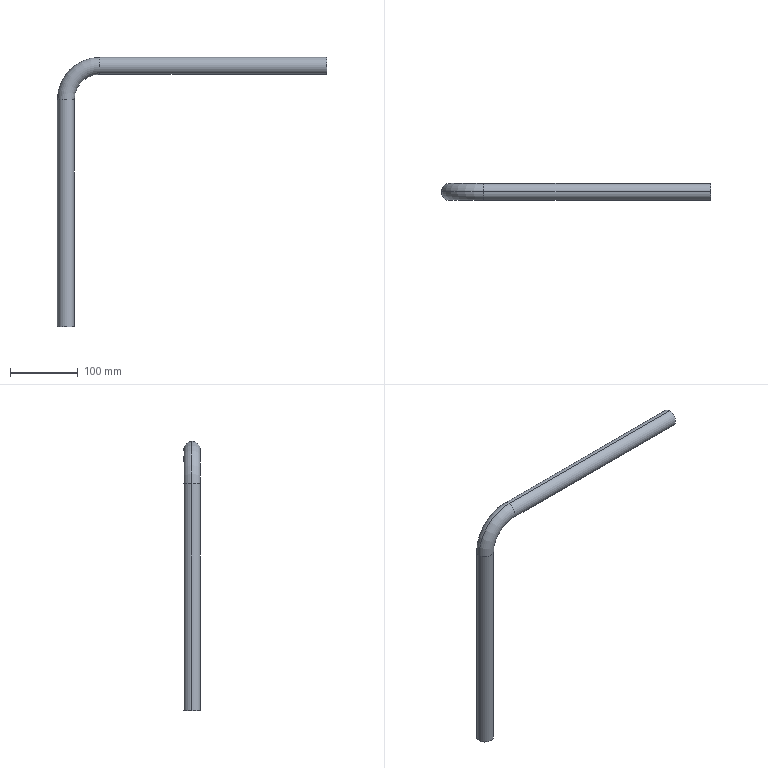Part | STEP file | 护栏90度栏杆_Default<As Machined> | 3 solids | 18 faces | box 397.5 x 25 x 397.5 mm | volume 82894 mm3 | cylinder 8 | plane 6 | torus 4 | commonest cylinder face diameters 22 x4 25 x4
STEP:
#1=CARTESIAN_POINT('',(0.,0.,0.));
#2=DIRECTION('',(0.,0.,1.));
#3=DIRECTION('',(1.,0.,0.));
#4=AXIS2_PLACEMENT_3D('',#1,#2,#3);
#5=CARTESIAN_POINT('',(50.,0.,12.5));
#6=VERTEX_POINT('',#5);
#7=CARTESIAN_POINT('',(50.,0.,-12.5));
#8=VERTEX_POINT('',#7);
#9=CARTESIAN_POINT('',(50.,0.,0.));
#10=DIRECTION('',(-1.,0.,0.));
#11=DIRECTION('',(0.,0.,1.));
#12=AXIS2_PLACEMENT_3D('',#9,#10,#11);
#13=CIRCLE('',#12,12.5);
#14=CARTESIAN_POINT('',(50.,0.,0.));
#15=DIRECTION('',(1.,0.,0.));
#16=DIRECTION('',(0.,0.,-1.));
#17=AXIS2_PLACEMENT_3D('',#14,#15,#16);
#18=CYLINDRICAL_SURFACE('',#17,12.5);
#19=CARTESIAN_POINT('',(3.142,0.));
#20=DIRECTION('',(-1.,0.));
#21=VECTOR('',#20,1.);
#22=LINE('',#19,#21);
#23=(GEOMETRIC_REPRESENTATION_CONTEXT(2)PARAMETRIC_REPRESENTATION_CONTEXT()REPRESENTATION_CONTEXT('',''));
#24=DEFINITIONAL_REPRESENTATION('',(#22),#23);
#25=PCURVE('',#18,#24);
#26=CARTESIAN_POINT('',(50.,0.,0.));
#27=DIRECTION('',(-1.,0.,0.));
#28=DIRECTION('',(0.,0.,1.));
#29=AXIS2_PLACEMENT_3D('',#26,#27,#28);
#30=PLANE('',#29);
#31=CARTESIAN_POINT('',(0.,0.));
#32=DIRECTION('',(1.,0.));
#33=AXIS2_PLACEMENT_2D('',#31,#32);
#34=CIRCLE('',#33,12.5);
#35=(GEOMETRIC_REPRESENTATION_CONTEXT(2)PARAMETRIC_REPRESENTATION_CONTEXT()REPRESENTATION_CONTEXT('',''));
#36=DEFINITIONAL_REPRESENTATION('',(#34),#35);
#37=PCURVE('',#30,#36);
#38=SURFACE_CURVE('',#13,(#25,#37),.PCURVE_S1.);
#39=EDGE_CURVE('',#6,#8,#38,.T.);
#40=ORIENTED_EDGE('',*,*,#39,.F.);
#41=CARTESIAN_POINT('',(385.,0.,12.5));
#42=VERTEX_POINT('',#41);
#43=CARTESIAN_POINT('',(50.,0.,12.5));
#44=DIRECTION('',(1.,0.,0.));
#45=VECTOR('',#44,1.);
#46=LINE('',#43,#45);
#47=CARTESIAN_POINT('',(3.142,0.));
#48=DIRECTION('',(0.,1.));
#49=VECTOR('',#48,1.);
#50=LINE('',#47,#49);
#51=(GEOMETRIC_REPRESENTATION_CONTEXT(2)PARAMETRIC_REPRESENTATION_CONTEXT()REPRESENTATION_CONTEXT('',''));
#52=DEFINITIONAL_REPRESENTATION('',(#50),#51);
#53=PCURVE('',#18,#52);
#54=CARTESIAN_POINT('',(50.,0.,0.));
#55=DIRECTION('',(1.,0.,0.));
#56=DIRECTION('',(0.,0.,-1.));
#57=AXIS2_PLACEMENT_3D('',#54,#55,#56);
#58=CYLINDRICAL_SURFACE('',#57,12.5);
#59=CARTESIAN_POINT('',(3.142,0.));
#60=DIRECTION('',(0.,1.));
#61=VECTOR('',#60,1.);
#62=LINE('',#59,#61);
#63=(GEOMETRIC_REPRESENTATION_CONTEXT(2)PARAMETRIC_REPRESENTATION_CONTEXT()REPRESENTATION_CONTEXT('',''));
#64=DEFINITIONAL_REPRESENTATION('',(#62),#63);
#65=PCURVE('',#58,#64);
#66=SURFACE_CURVE('',#46,(#53,#65),.PCURVE_S1.);
#67=EDGE_CURVE('',#6,#42,#66,.T.);
#68=ORIENTED_EDGE('',*,*,#67,.T.);
#69=CARTESIAN_POINT('',(385.,0.,-12.5));
#70=VERTEX_POINT('',#69);
#71=CARTESIAN_POINT('',(385.,0.,0.));
#72=DIRECTION('',(-1.,0.,0.));
#73=DIRECTION('',(0.,0.,1.));
#74=AXIS2_PLACEMENT_3D('',#71,#72,#73);
#75=CIRCLE('',#74,12.5);
#76=CARTESIAN_POINT('',(3.142,335.));
#77=DIRECTION('',(-1.,0.));
#78=VECTOR('',#77,1.);
#79=LINE('',#76,#78);
#80=(GEOMETRIC_REPRESENTATION_CONTEXT(2)PARAMETRIC_REPRESENTATION_CONTEXT()REPRESENTATION_CONTEXT('',''));
#81=DEFINITIONAL_REPRESENTATION('',(#79),#80);
#82=PCURVE('',#18,#81);
#83=CARTESIAN_POINT('',(385.,0.,0.));
#84=DIRECTION('',(-1.,0.,0.));
#85=DIRECTION('',(0.,0.,1.));
#86=AXIS2_PLACEMENT_3D('',#83,#84,#85);
#87=PLANE('',#86);
#88=CARTESIAN_POINT('',(0.,0.));
#89=DIRECTION('',(1.,0.));
#90=AXIS2_PLACEMENT_2D('',#88,#89);
#91=CIRCLE('',#90,12.5);
#92=(GEOMETRIC_REPRESENTATION_CONTEXT(2)PARAMETRIC_REPRESENTATION_CONTEXT()REPRESENTATION_CONTEXT('',''));
#93=DEFINITIONAL_REPRESENTATION('',(#91),#92);
#94=PCURVE('',#87,#93);
#95=SURFACE_CURVE('',#75,(#82,#94),.PCURVE_S1.);
#96=EDGE_CURVE('',#42,#70,#95,.T.);
#97=ORIENTED_EDGE('',*,*,#96,.T.);
#98=CARTESIAN_POINT('',(50.,0.,-12.5));
#99=DIRECTION('',(1.,0.,0.));
#100=VECTOR('',#99,1.);
#101=LINE('',#98,#100);
#102=CARTESIAN_POINT('',(0.,0.));
#103=DIRECTION('',(0.,1.));
#104=VECTOR('',#103,1.);
#105=LINE('',#102,#104);
#106=(GEOMETRIC_REPRESENTATION_CONTEXT(2)PARAMETRIC_REPRESENTATION_CONTEXT()REPRESENTATION_CONTEXT('',''));
#107=DEFINITIONAL_REPRESENTATION('',(#105),#106);
#108=PCURVE('',#18,#107);
#109=CARTESIAN_POINT('',(6.283,0.));
#110=DIRECTION('',(0.,1.));
#111=VECTOR('',#110,1.);
#112=LINE('',#109,#111);
#113=(GEOMETRIC_REPRESENTATION_CONTEXT(2)PARAMETRIC_REPRESENTATION_CONTEXT()REPRESENTATION_CONTEXT('',''));
#114=DEFINITIONAL_REPRESENTATION('',(#112),#113);
#115=PCURVE('',#58,#114);
#116=SURFACE_CURVE('',#101,(#108,#115),.PCURVE_S1.);
#117=EDGE_CURVE('',#8,#70,#116,.T.);
#118=ORIENTED_EDGE('',*,*,#117,.F.);
#119=EDGE_LOOP('',(#40,#68,#97,#118));
#120=FACE_BOUND('',#119,.T.);
#121=ADVANCED_FACE('',(#120),#18,.T.);
#122=CARTESIAN_POINT('',(50.,0.,-11.));
#123=VERTEX_POINT('',#122);
#124=CARTESIAN_POINT('',(385.,0.,-11.));
#125=VERTEX_POINT('',#124);
#126=CARTESIAN_POINT('',(50.,0.,-11.));
#127=DIRECTION('',(1.,0.,0.));
#128=VECTOR('',#127,1.);
#129=LINE('',#126,#128);
#130=CARTESIAN_POINT('',(50.,0.,0.));
#131=DIRECTION('',(1.,0.,0.));
#132=DIRECTION('',(0.,0.,-1.));
#133=AXIS2_PLACEMENT_3D('',#130,#131,#132);
#134=CYLINDRICAL_SURFACE('',#133,11.);
#135=CARTESIAN_POINT('',(6.283,0.));
#136=DIRECTION('',(0.,1.));
#137=VECTOR('',#136,1.);
#138=LINE('',#135,#137);
#139=(GEOMETRIC_REPRESENTATION_CONTEXT(2)PARAMETRIC_REPRESENTATION_CONTEXT()REPRESENTATION_CONTEXT('',''));
#140=DEFINITIONAL_REPRESENTATION('',(#138),#139);
#141=PCURVE('',#134,#140);
#142=CARTESIAN_POINT('',(50.,0.,0.));
#143=DIRECTION('',(1.,0.,0.));
#144=DIRECTION('',(0.,0.,-1.));
#145=AXIS2_PLACEMENT_3D('',#142,#143,#144);
#146=CYLINDRICAL_SURFACE('',#145,11.);
#147=CARTESIAN_POINT('',(0.,0.));
#148=DIRECTION('',(0.,1.));
#149=VECTOR('',#148,1.);
#150=LINE('',#147,#149);
#151=(GEOMETRIC_REPRESENTATION_CONTEXT(2)PARAMETRIC_REPRESENTATION_CONTEXT()REPRESENTATION_CONTEXT('',''));
#152=DEFINITIONAL_REPRESENTATION('',(#150),#151);
#153=PCURVE('',#146,#152);
#154=SURFACE_CURVE('',#129,(#141,#153),.PCURVE_S1.);
#155=EDGE_CURVE('',#123,#125,#154,.T.);
#156=ORIENTED_EDGE('',*,*,#155,.T.);
#157=CARTESIAN_POINT('',(385.,0.,11.));
#158=VERTEX_POINT('',#157);
#159=CARTESIAN_POINT('',(385.,0.,0.));
#160=DIRECTION('',(-1.,0.,0.));
#161=DIRECTION('',(0.,0.,1.));
#162=AXIS2_PLACEMENT_3D('',#159,#160,#161);
#163=CIRCLE('',#162,11.);
#164=CARTESIAN_POINT('',(9.425,335.));
#165=DIRECTION('',(-1.,0.));
#166=VECTOR('',#165,1.);
#167=LINE('',#164,#166);
#168=(GEOMETRIC_REPRESENTATION_CONTEXT(2)PARAMETRIC_REPRESENTATION_CONTEXT()REPRESENTATION_CONTEXT('',''));
#169=DEFINITIONAL_REPRESENTATION('',(#167),#168);
#170=PCURVE('',#134,#169);
#171=CARTESIAN_POINT('',(0.,0.));
#172=DIRECTION('',(1.,0.));
#173=AXIS2_PLACEMENT_2D('',#171,#172);
#174=CIRCLE('',#173,11.);
#175=(GEOMETRIC_REPRESENTATION_CONTEXT(2)PARAMETRIC_REPRESENTATION_CONTEXT()REPRESENTATION_CONTEXT('',''));
#176=DEFINITIONAL_REPRESENTATION('',(#174),#175);
#177=PCURVE('',#87,#176);
#178=SURFACE_CURVE('',#163,(#170,#177),.PCURVE_S1.);
#179=EDGE_CURVE('',#125,#158,#178,.T.);
#180=ORIENTED_EDGE('',*,*,#179,.T.);
#181=CARTESIAN_POINT('',(50.,0.,11.));
#182=VERTEX_POINT('',#181);
#183=CARTESIAN_POINT('',(50.,0.,11.));
#184=DIRECTION('',(1.,0.,0.));
#185=VECTOR('',#184,1.);
#186=LINE('',#183,#185);
#187=CARTESIAN_POINT('',(3.142,0.));
#188=DIRECTION('',(0.,1.));
#189=VECTOR('',#188,1.);
#190=LINE('',#187,#189);
#191=(GEOMETRIC_REPRESENTATION_CONTEXT(2)PARAMETRIC_REPRESENTATION_CONTEXT()REPRESENTATION_CONTEXT('',''));
#192=DEFINITIONAL_REPRESENTATION('',(#190),#191);
#193=PCURVE('',#134,#192);
#194=CARTESIAN_POINT('',(3.142,0.));
#195=DIRECTION('',(0.,1.));
#196=VECTOR('',#195,1.);
#197=LINE('',#194,#196);
#198=(GEOMETRIC_REPRESENTATION_CONTEXT(2)PARAMETRIC_REPRESENTATION_CONTEXT()REPRESENTATION_CONTEXT('',''));
#199=DEFINITIONAL_REPRESENTATION('',(#197),#198);
#200=PCURVE('',#146,#199);
#201=SURFACE_CURVE('',#186,(#193,#200),.PCURVE_S1.);
#202=EDGE_CURVE('',#182,#158,#201,.T.);
#203=ORIENTED_EDGE('',*,*,#202,.F.);
#204=CARTESIAN_POINT('',(50.,0.,0.));
#205=DIRECTION('',(-1.,0.,0.));
#206=DIRECTION('',(0.,0.,1.));
#207=AXIS2_PLACEMENT_3D('',#204,#205,#206);
#208=CIRCLE('',#207,11.);
#209=CARTESIAN_POINT('',(9.425,0.));
#210=DIRECTION('',(-1.,0.));
#211=VECTOR('',#210,1.);
#212=LINE('',#209,#211);
#213=(GEOMETRIC_REPRESENTATION_CONTEXT(2)PARAMETRIC_REPRESENTATION_CONTEXT()REPRESENTATION_CONTEXT('',''));
#214=DEFINITIONAL_REPRESENTATION('',(#212),#213);
#215=PCURVE('',#134,#214);
#216=CARTESIAN_POINT('',(0.,0.));
#217=DIRECTION('',(1.,0.));
#218=AXIS2_PLACEMENT_2D('',#216,#217);
#219=CIRCLE('',#218,11.);
#220=(GEOMETRIC_REPRESENTATION_CONTEXT(2)PARAMETRIC_REPRESENTATION_CONTEXT()REPRESENTATION_CONTEXT('',''));
#221=DEFINITIONAL_REPRESENTATION('',(#219),#220);
#222=PCURVE('',#30,#221);
#223=SURFACE_CURVE('',#208,(#215,#222),.PCURVE_S1.);
#224=EDGE_CURVE('',#123,#182,#223,.T.);
#225=ORIENTED_EDGE('',*,*,#224,.F.);
#226=EDGE_LOOP('',(#156,#180,#203,#225));
#227=FACE_BOUND('',#226,.F.);
#228=ADVANCED_FACE('',(#227),#134,.F.);
#229=CARTESIAN_POINT('',(385.,0.,0.));
#230=DIRECTION('',(-1.,0.,0.));
#231=DIRECTION('',(0.,0.,1.));
#232=AXIS2_PLACEMENT_3D('',#229,#230,#231);
#233=CIRCLE('',#232,11.);
#234=CARTESIAN_POINT('',(3.142,335.));
#235=DIRECTION('',(-1.,0.));
#236=VECTOR('',#235,1.);
#237=LINE('',#234,#236);
#238=(GEOMETRIC_REPRESENTATION_CONTEXT(2)PARAMETRIC_REPRESENTATION_CONTEXT()REPRESENTATION_CONTEXT('',''));
#239=DEFINITIONAL_REPRESENTATION('',(#237),#238);
#240=PCURVE('',#146,#239);
#241=CARTESIAN_POINT('',(0.,0.));
#242=DIRECTION('',(1.,0.));
#243=AXIS2_PLACEMENT_2D('',#241,#242);
#244=CIRCLE('',#243,11.);
#245=(GEOMETRIC_REPRESENTATION_CONTEXT(2)PARAMETRIC_REPRESENTATION_CONTEXT()REPRESENTATION_CONTEXT('',''));
#246=DEFINITIONAL_REPRESENTATION('',(#244),#245);
#247=PCURVE('',#87,#246);
#248=SURFACE_CURVE('',#233,(#240,#247),.PCURVE_S1.);
#249=EDGE_CURVE('',#158,#125,#248,.T.);
#250=ORIENTED_EDGE('',*,*,#249,.T.);
#251=ORIENTED_EDGE('',*,*,#155,.F.);
#252=CARTESIAN_POINT('',(50.,0.,0.));
#253=DIRECTION('',(-1.,0.,0.));
#254=DIRECTION('',(0.,0.,1.));
#255=AXIS2_PLACEMENT_3D('',#252,#253,#254);
#256=CIRCLE('',#255,11.);
#257=CARTESIAN_POINT('',(3.142,0.));
#258=DIRECTION('',(-1.,0.));
#259=VECTOR('',#258,1.);
#260=LINE('',#257,#259);
#261=(GEOMETRIC_REPRESENTATION_CONTEXT(2)PARAMETRIC_REPRESENTATION_CONTEXT()REPRESENTATION_CONTEXT('',''));
#262=DEFINITIONAL_REPRESENTATION('',(#260),#261);
#263=PCURVE('',#146,#262);
#264=CARTESIAN_POINT('',(0.,0.));
#265=DIRECTION('',(1.,0.));
#266=AXIS2_PLACEMENT_2D('',#264,#265);
#267=CIRCLE('',#266,11.);
#268=(GEOMETRIC_REPRESENTATION_CONTEXT(2)PARAMETRIC_REPRESENTATION_CONTEXT()REPRESENTATION_CONTEXT('',''));
#269=DEFINITIONAL_REPRESENTATION('',(#267),#268);
#270=PCURVE('',#30,#269);
#271=SURFACE_CURVE('',#256,(#263,#270),.PCURVE_S1.);
#272=EDGE_CURVE('',#182,#123,#271,.T.);
#273=ORIENTED_EDGE('',*,*,#272,.F.);
#274=ORIENTED_EDGE('',*,*,#202,.T.);
#275=EDGE_LOOP('',(#250,#251,#273,#274));
#276=FACE_BOUND('',#275,.F.);
#277=ADVANCED_FACE('',(#276),#146,.F.);
#278=ORIENTED_EDGE('',*,*,#67,.F.);
#279=CARTESIAN_POINT('',(50.,0.,0.));
#280=DIRECTION('',(-1.,0.,0.));
#281=DIRECTION('',(0.,0.,1.));
#282=AXIS2_PLACEMENT_3D('',#279,#280,#281);
#283=CIRCLE('',#282,12.5);
#284=CARTESIAN_POINT('',(9.425,0.));
#285=DIRECTION('',(-1.,0.));
#286=VECTOR('',#285,1.);
#287=LINE('',#284,#286);
#288=(GEOMETRIC_REPRESENTATION_CONTEXT(2)PARAMETRIC_REPRESENTATION_CONTEXT()REPRESENTATION_CONTEXT('',''));
#289=DEFINITIONAL_REPRESENTATION('',(#287),#288);
#290=PCURVE('',#58,#289);
#291=CARTESIAN_POINT('',(0.,0.));
#292=DIRECTION('',(1.,0.));
#293=AXIS2_PLACEMENT_2D('',#291,#292);
#294=CIRCLE('',#293,12.5);
#295=(GEOMETRIC_REPRESENTATION_CONTEXT(2)PARAMETRIC_REPRESENTATION_CONTEXT()REPRESENTATION_CONTEXT('',''));
#296=DEFINITIONAL_REPRESENTATION('',(#294),#295);
#297=PCURVE('',#30,#296);
#298=SURFACE_CURVE('',#283,(#290,#297),.PCURVE_S1.);
#299=EDGE_CURVE('',#8,#6,#298,.T.);
#300=ORIENTED_EDGE('',*,*,#299,.F.);
#301=ORIENTED_EDGE('',*,*,#117,.T.);
#302=CARTESIAN_POINT('',(385.,0.,0.));
#303=DIRECTION('',(-1.,0.,0.));
#304=DIRECTION('',(0.,0.,1.));
#305=AXIS2_PLACEMENT_3D('',#302,#303,#304);
#306=CIRCLE('',#305,12.5);
#307=CARTESIAN_POINT('',(9.425,335.));
#308=DIRECTION('',(-1.,0.));
#309=VECTOR('',#308,1.);
#310=LINE('',#307,#309);
#311=(GEOMETRIC_REPRESENTATION_CONTEXT(2)PARAMETRIC_REPRESENTATION_CONTEXT()REPRESENTATION_CONTEXT('',''));
#312=DEFINITIONAL_REPRESENTATION('',(#310),#311);
#313=PCURVE('',#58,#312);
#314=CARTESIAN_POINT('',(0.,0.));
#315=DIRECTION('',(1.,0.));
#316=AXIS2_PLACEMENT_2D('',#314,#315);
#317=CIRCLE('',#316,12.5);
#318=(GEOMETRIC_REPRESENTATION_CONTEXT(2)PARAMETRIC_REPRESENTATION_CONTEXT()REPRESENTATION_CONTEXT('',''));
#319=DEFINITIONAL_REPRESENTATION('',(#317),#318);
#320=PCURVE('',#87,#319);
#321=SURFACE_CURVE('',#306,(#313,#320),.PCURVE_S1.);
#322=EDGE_CURVE('',#70,#42,#321,.T.);
#323=ORIENTED_EDGE('',*,*,#322,.T.);
#324=EDGE_LOOP('',(#278,#300,#301,#323));
#325=FACE_BOUND('',#324,.T.);
#326=ADVANCED_FACE('',(#325),#58,.T.);
#327=ORIENTED_EDGE('',*,*,#179,.T.);
#328=ORIENTED_EDGE('',*,*,#249,.T.);
#329=EDGE_LOOP('',(#327,#328));
#330=FACE_BOUND('',#329,.T.);
#331=ORIENTED_EDGE('',*,*,#322,.F.);
#332=ORIENTED_EDGE('',*,*,#96,.F.);
#333=EDGE_LOOP('',(#331,#332));
#334=FACE_BOUND('',#333,.T.);
#335=ADVANCED_FACE('',(#330,#334),#87,.F.);
#336=ORIENTED_EDGE('',*,*,#224,.F.);
#337=ORIENTED_EDGE('',*,*,#272,.F.);
#338=EDGE_LOOP('',(#336,#337));
#339=FACE_BOUND('',#338,.T.);
#340=ORIENTED_EDGE('',*,*,#299,.T.);
#341=ORIENTED_EDGE('',*,*,#39,.T.);
#342=EDGE_LOOP('',(#340,#341));
#343=FACE_BOUND('',#342,.T.);
#344=ADVANCED_FACE('',(#339,#343),#30,.T.);
#345=CLOSED_SHELL('',(#121,#228,#277,#326,#335,#344));
#346=MANIFOLD_SOLID_BREP('',#345);
#347=CARTESIAN_POINT('',(-12.5,0.,-50.));
#348=VERTEX_POINT('',#347);
#349=CARTESIAN_POINT('',(12.5,0.,-50.));
#350=VERTEX_POINT('',#349);
#351=CARTESIAN_POINT('',(0.,0.,-50.));
#352=DIRECTION('',(0.,0.,-1.));
#353=DIRECTION('',(-1.,0.,0.));
#354=AXIS2_PLACEMENT_3D('',#351,#352,#353);
#355=CIRCLE('',#354,12.5);
#356=CARTESIAN_POINT('',(50.,0.,-50.));
#357=DIRECTION('',(0.,1.,0.));
#358=DIRECTION('',(0.,0.,1.));
#359=AXIS2_PLACEMENT_3D('',#356,#357,#358);
#360=TOROIDAL_SURFACE('',#359,50.,12.5);
#361=CARTESIAN_POINT('',(4.712,0.));
#362=DIRECTION('',(0.,1.));
#363=VECTOR('',#362,1.);
#364=LINE('',#361,#363);
#365=(GEOMETRIC_REPRESENTATION_CONTEXT(2)PARAMETRIC_REPRESENTATION_CONTEXT()REPRESENTATION_CONTEXT('',''));
#366=DEFINITIONAL_REPRESENTATION('',(#364),#365);
#367=PCURVE('',#360,#366);
#368=CARTESIAN_POINT('',(0.,0.,-50.));
#369=DIRECTION('',(0.,0.,-1.));
#370=DIRECTION('',(-1.,0.,0.));
#371=AXIS2_PLACEMENT_3D('',#368,#369,#370);
#372=PLANE('',#371);
#373=CARTESIAN_POINT('',(0.,0.));
#374=DIRECTION('',(1.,0.));
#375=AXIS2_PLACEMENT_2D('',#373,#374);
#376=CIRCLE('',#375,12.5);
#377=(GEOMETRIC_REPRESENTATION_CONTEXT(2)PARAMETRIC_REPRESENTATION_CONTEXT()REPRESENTATION_CONTEXT('',''));
#378=DEFINITIONAL_REPRESENTATION('',(#376),#377);
#379=PCURVE('',#372,#378);
#380=SURFACE_CURVE('',#355,(#367,#379),.PCURVE_S1.);
#381=EDGE_CURVE('',#348,#350,#380,.T.);
#382=ORIENTED_EDGE('',*,*,#381,.F.);
#383=CARTESIAN_POINT('',(50.,0.,12.5));
#384=VERTEX_POINT('',#383);
#385=CARTESIAN_POINT('',(50.,0.,-50.));
#386=DIRECTION('',(0.,1.,0.));
#387=DIRECTION('',(0.,0.,1.));
#388=AXIS2_PLACEMENT_3D('',#385,#386,#387);
#389=CIRCLE('',#388,62.5);
#390=CARTESIAN_POINT('',(0.,0.));
#391=DIRECTION('',(1.,0.));
#392=VECTOR('',#391,1.);
#393=LINE('',#390,#392);
#394=(GEOMETRIC_REPRESENTATION_CONTEXT(2)PARAMETRIC_REPRESENTATION_CONTEXT()REPRESENTATION_CONTEXT('',''));
#395=DEFINITIONAL_REPRESENTATION('',(#393),#394);
#396=PCURVE('',#360,#395);
#397=CARTESIAN_POINT('',(50.,0.,-50.));
#398=DIRECTION('',(0.,1.,0.));
#399=DIRECTION('',(0.,0.,1.));
#400=AXIS2_PLACEMENT_3D('',#397,#398,#399);
#401=TOROIDAL_SURFACE('',#400,50.,12.5);
#402=CARTESIAN_POINT('',(0.,6.283));
#403=DIRECTION('',(1.,0.));
#404=VECTOR('',#403,1.);
#405=LINE('',#402,#404);
#406=(GEOMETRIC_REPRESENTATION_CONTEXT(2)PARAMETRIC_REPRESENTATION_CONTEXT()REPRESENTATION_CONTEXT('',''));
#407=DEFINITIONAL_REPRESENTATION('',(#405),#406);
#408=PCURVE('',#401,#407);
#409=SURFACE_CURVE('',#389,(#396,#408),.PCURVE_S1.);
#410=EDGE_CURVE('',#348,#384,#409,.T.);
#411=ORIENTED_EDGE('',*,*,#410,.T.);
#412=CARTESIAN_POINT('',(50.,0.,-12.5));
#413=VERTEX_POINT('',#412);
#414=CARTESIAN_POINT('',(50.,0.,0.));
#415=DIRECTION('',(1.,0.,0.));
#416=DIRECTION('',(0.,0.,-1.));
#417=AXIS2_PLACEMENT_3D('',#414,#415,#416);
#418=CIRCLE('',#417,12.5);
#419=CARTESIAN_POINT('',(6.283,3.142));
#420=DIRECTION('',(0.,-1.));
#421=VECTOR('',#420,1.);
#422=LINE('',#419,#421);
#423=(GEOMETRIC_REPRESENTATION_CONTEXT(2)PARAMETRIC_REPRESENTATION_CONTEXT()REPRESENTATION_CONTEXT('',''));
#424=DEFINITIONAL_REPRESENTATION('',(#422),#423);
#425=PCURVE('',#360,#424);
#426=CARTESIAN_POINT('',(50.,0.,0.));
#427=DIRECTION('',(1.,0.,0.));
#428=DIRECTION('',(0.,0.,-1.));
#429=AXIS2_PLACEMENT_3D('',#426,#427,#428);
#430=PLANE('',#429);
#431=CARTESIAN_POINT('',(0.,0.));
#432=DIRECTION('',(1.,0.));
#433=AXIS2_PLACEMENT_2D('',#431,#432);
#434=CIRCLE('',#433,12.5);
#435=(GEOMETRIC_REPRESENTATION_CONTEXT(2)PARAMETRIC_REPRESENTATION_CONTEXT()REPRESENTATION_CONTEXT('',''));
#436=DEFINITIONAL_REPRESENTATION('',(#434),#435);
#437=PCURVE('',#430,#436);
#438=SURFACE_CURVE('',#418,(#425,#437),.PCURVE_S1.);
#439=EDGE_CURVE('',#413,#384,#438,.T.);
#440=ORIENTED_EDGE('',*,*,#439,.F.);
#441=CARTESIAN_POINT('',(50.,0.,-50.));
#442=DIRECTION('',(0.,1.,0.));
#443=DIRECTION('',(0.,0.,1.));
#444=AXIS2_PLACEMENT_3D('',#441,#442,#443);
#445=CIRCLE('',#444,37.5);
#446=CARTESIAN_POINT('',(0.,3.142));
#447=DIRECTION('',(1.,0.));
#448=VECTOR('',#447,1.);
#449=LINE('',#446,#448);
#450=(GEOMETRIC_REPRESENTATION_CONTEXT(2)PARAMETRIC_REPRESENTATION_CONTEXT()REPRESENTATION_CONTEXT('',''));
#451=DEFINITIONAL_REPRESENTATION('',(#449),#450);
#452=PCURVE('',#360,#451);
#453=CARTESIAN_POINT('',(0.,3.142));
#454=DIRECTION('',(1.,0.));
#455=VECTOR('',#454,1.);
#456=LINE('',#453,#455);
#457=(GEOMETRIC_REPRESENTATION_CONTEXT(2)PARAMETRIC_REPRESENTATION_CONTEXT()REPRESENTATION_CONTEXT('',''));
#458=DEFINITIONAL_REPRESENTATION('',(#456),#457);
#459=PCURVE('',#401,#458);
#460=SURFACE_CURVE('',#445,(#452,#459),.PCURVE_S1.);
#461=EDGE_CURVE('',#350,#413,#460,.T.);
#462=ORIENTED_EDGE('',*,*,#461,.F.);
#463=EDGE_LOOP('',(#382,#411,#440,#462));
#464=FACE_BOUND('',#463,.T.);
#465=ADVANCED_FACE('',(#464),#360,.T.);
#466=CARTESIAN_POINT('',(11.,0.,-50.));
#467=VERTEX_POINT('',#466);
#468=CARTESIAN_POINT('',(50.,0.,-11.));
#469=VERTEX_POINT('',#468);
#470=CARTESIAN_POINT('',(50.,0.,-50.));
#471=DIRECTION('',(0.,1.,0.));
#472=DIRECTION('',(0.,0.,1.));
#473=AXIS2_PLACEMENT_3D('',#470,#471,#472);
#474=CIRCLE('',#473,39.);
#475=CARTESIAN_POINT('',(50.,0.,-50.));
#476=DIRECTION('',(0.,1.,0.));
#477=DIRECTION('',(0.,0.,1.));
#478=AXIS2_PLACEMENT_3D('',#475,#476,#477);
#479=TOROIDAL_SURFACE('',#478,50.,11.);
#480=CARTESIAN_POINT('',(0.,3.142));
#481=DIRECTION('',(1.,0.));
#482=VECTOR('',#481,1.);
#483=LINE('',#480,#482);
#484=(GEOMETRIC_REPRESENTATION_CONTEXT(2)PARAMETRIC_REPRESENTATION_CONTEXT()REPRESENTATION_CONTEXT('',''));
#485=DEFINITIONAL_REPRESENTATION('',(#483),#484);
#486=PCURVE('',#479,#485);
#487=CARTESIAN_POINT('',(50.,0.,-50.));
#488=DIRECTION('',(0.,1.,0.));
#489=DIRECTION('',(0.,0.,1.));
#490=AXIS2_PLACEMENT_3D('',#487,#488,#489);
#491=TOROIDAL_SURFACE('',#490,50.,11.);
#492=CARTESIAN_POINT('',(0.,3.142));
#493=DIRECTION('',(1.,0.));
#494=VECTOR('',#493,1.);
#495=LINE('',#492,#494);
#496=(GEOMETRIC_REPRESENTATION_CONTEXT(2)PARAMETRIC_REPRESENTATION_CONTEXT()REPRESENTATION_CONTEXT('',''));
#497=DEFINITIONAL_REPRESENTATION('',(#495),#496);
#498=PCURVE('',#491,#497);
#499=SURFACE_CURVE('',#474,(#486,#498),.PCURVE_S1.);
#500=EDGE_CURVE('',#467,#469,#499,.T.);
#501=ORIENTED_EDGE('',*,*,#500,.T.);
#502=CARTESIAN_POINT('',(50.,0.,11.));
#503=VERTEX_POINT('',#502);
#504=CARTESIAN_POINT('',(50.,0.,0.));
#505=DIRECTION('',(1.,0.,0.));
#506=DIRECTION('',(0.,0.,-1.));
#507=AXIS2_PLACEMENT_3D('',#504,#505,#506);
#508=CIRCLE('',#507,11.);
#509=CARTESIAN_POINT('',(6.283,9.425));
#510=DIRECTION('',(0.,-1.));
#511=VECTOR('',#510,1.);
#512=LINE('',#509,#511);
#513=(GEOMETRIC_REPRESENTATION_CONTEXT(2)PARAMETRIC_REPRESENTATION_CONTEXT()REPRESENTATION_CONTEXT('',''));
#514=DEFINITIONAL_REPRESENTATION('',(#512),#513);
#515=PCURVE('',#479,#514);
#516=CARTESIAN_POINT('',(0.,0.));
#517=DIRECTION('',(1.,0.));
#518=AXIS2_PLACEMENT_2D('',#516,#517);
#519=CIRCLE('',#518,11.);
#520=(GEOMETRIC_REPRESENTATION_CONTEXT(2)PARAMETRIC_REPRESENTATION_CONTEXT()REPRESENTATION_CONTEXT('',''));
#521=DEFINITIONAL_REPRESENTATION('',(#519),#520);
#522=PCURVE('',#430,#521);
#523=SURFACE_CURVE('',#508,(#515,#522),.PCURVE_S1.);
#524=EDGE_CURVE('',#503,#469,#523,.T.);
#525=ORIENTED_EDGE('',*,*,#524,.F.);
#526=CARTESIAN_POINT('',(-11.,0.,-50.));
#527=VERTEX_POINT('',#526);
#528=CARTESIAN_POINT('',(50.,0.,-50.));
#529=DIRECTION('',(0.,1.,0.));
#530=DIRECTION('',(0.,0.,1.));
#531=AXIS2_PLACEMENT_3D('',#528,#529,#530);
#532=CIRCLE('',#531,61.);
#533=CARTESIAN_POINT('',(0.,6.283));
#534=DIRECTION('',(1.,0.));
#535=VECTOR('',#534,1.);
#536=LINE('',#533,#535);
#537=(GEOMETRIC_REPRESENTATION_CONTEXT(2)PARAMETRIC_REPRESENTATION_CONTEXT()REPRESENTATION_CONTEXT('',''));
#538=DEFINITIONAL_REPRESENTATION('',(#536),#537);
#539=PCURVE('',#479,#538);
#540=CARTESIAN_POINT('',(0.,0.));
#541=DIRECTION('',(1.,0.));
#542=VECTOR('',#541,1.);
#543=LINE('',#540,#542);
#544=(GEOMETRIC_REPRESENTATION_CONTEXT(2)PARAMETRIC_REPRESENTATION_CONTEXT()REPRESENTATION_CONTEXT('',''));
#545=DEFINITIONAL_REPRESENTATION('',(#543),#544);
#546=PCURVE('',#491,#545);
#547=SURFACE_CURVE('',#532,(#539,#546),.PCURVE_S1.);
#548=EDGE_CURVE('',#527,#503,#547,.T.);
#549=ORIENTED_EDGE('',*,*,#548,.F.);
#550=CARTESIAN_POINT('',(0.,0.,-50.));
#551=DIRECTION('',(0.,0.,-1.));
#552=DIRECTION('',(-1.,0.,0.));
#553=AXIS2_PLACEMENT_3D('',#550,#551,#552);
#554=CIRCLE('',#553,11.);
#555=CARTESIAN_POINT('',(4.712,0.));
#556=DIRECTION('',(0.,1.));
#557=VECTOR('',#556,1.);
#558=LINE('',#555,#557);
#559=(GEOMETRIC_REPRESENTATION_CONTEXT(2)PARAMETRIC_REPRESENTATION_CONTEXT()REPRESENTATION_CONTEXT('',''));
#560=DEFINITIONAL_REPRESENTATION('',(#558),#559);
#561=PCURVE('',#479,#560);
#562=CARTESIAN_POINT('',(0.,0.));
#563=DIRECTION('',(1.,0.));
#564=AXIS2_PLACEMENT_2D('',#562,#563);
#565=CIRCLE('',#564,11.);
#566=(GEOMETRIC_REPRESENTATION_CONTEXT(2)PARAMETRIC_REPRESENTATION_CONTEXT()REPRESENTATION_CONTEXT('',''));
#567=DEFINITIONAL_REPRESENTATION('',(#565),#566);
#568=PCURVE('',#372,#567);
#569=SURFACE_CURVE('',#554,(#561,#568),.PCURVE_S1.);
#570=EDGE_CURVE('',#467,#527,#569,.T.);
#571=ORIENTED_EDGE('',*,*,#570,.F.);
#572=EDGE_LOOP('',(#501,#525,#549,#571));
#573=FACE_BOUND('',#572,.F.);
#574=ADVANCED_FACE('',(#573),#479,.F.);
#575=CARTESIAN_POINT('',(50.,0.,0.));
#576=DIRECTION('',(1.,0.,0.));
#577=DIRECTION('',(0.,0.,-1.));
#578=AXIS2_PLACEMENT_3D('',#575,#576,#577);
#579=CIRCLE('',#578,11.);
#580=CARTESIAN_POINT('',(6.283,3.142));
#581=DIRECTION('',(0.,-1.));
#582=VECTOR('',#581,1.);
#583=LINE('',#580,#582);
#584=(GEOMETRIC_REPRESENTATION_CONTEXT(2)PARAMETRIC_REPRESENTATION_CONTEXT()REPRESENTATION_CONTEXT('',''));
#585=DEFINITIONAL_REPRESENTATION('',(#583),#584);
#586=PCURVE('',#491,#585);
#587=CARTESIAN_POINT('',(0.,0.));
#588=DIRECTION('',(1.,0.));
#589=AXIS2_PLACEMENT_2D('',#587,#588);
#590=CIRCLE('',#589,11.);
#591=(GEOMETRIC_REPRESENTATION_CONTEXT(2)PARAMETRIC_REPRESENTATION_CONTEXT()REPRESENTATION_CONTEXT('',''));
#592=DEFINITIONAL_REPRESENTATION('',(#590),#591);
#593=PCURVE('',#430,#592);
#594=SURFACE_CURVE('',#579,(#586,#593),.PCURVE_S1.);
#595=EDGE_CURVE('',#469,#503,#594,.T.);
#596=ORIENTED_EDGE('',*,*,#595,.F.);
#597=ORIENTED_EDGE('',*,*,#500,.F.);
#598=CARTESIAN_POINT('',(0.,0.,-50.));
#599=DIRECTION('',(0.,0.,-1.));
#600=DIRECTION('',(-1.,0.,0.));
#601=AXIS2_PLACEMENT_3D('',#598,#599,#600);
#602=CIRCLE('',#601,11.);
#603=CARTESIAN_POINT('',(4.712,0.));
#604=DIRECTION('',(0.,1.));
#605=VECTOR('',#604,1.);
#606=LINE('',#603,#605);
#607=(GEOMETRIC_REPRESENTATION_CONTEXT(2)PARAMETRIC_REPRESENTATION_CONTEXT()REPRESENTATION_CONTEXT('',''));
#608=DEFINITIONAL_REPRESENTATION('',(#606),#607);
#609=PCURVE('',#491,#608);
#610=CARTESIAN_POINT('',(0.,0.));
#611=DIRECTION('',(1.,0.));
#612=AXIS2_PLACEMENT_2D('',#610,#611);
#613=CIRCLE('',#612,11.);
#614=(GEOMETRIC_REPRESENTATION_CONTEXT(2)PARAMETRIC_REPRESENTATION_CONTEXT()REPRESENTATION_CONTEXT('',''));
#615=DEFINITIONAL_REPRESENTATION('',(#613),#614);
#616=PCURVE('',#372,#615);
#617=SURFACE_CURVE('',#602,(#609,#616),.PCURVE_S1.);
#618=EDGE_CURVE('',#527,#467,#617,.T.);
#619=ORIENTED_EDGE('',*,*,#618,.F.);
#620=ORIENTED_EDGE('',*,*,#548,.T.);
#621=EDGE_LOOP('',(#596,#597,#619,#620));
#622=FACE_BOUND('',#621,.F.);
#623=ADVANCED_FACE('',(#622),#491,.F.);
#624=ORIENTED_EDGE('',*,*,#410,.F.);
#625=CARTESIAN_POINT('',(0.,0.,-50.));
#626=DIRECTION('',(0.,0.,-1.));
#627=DIRECTION('',(-1.,0.,0.));
#628=AXIS2_PLACEMENT_3D('',#625,#626,#627);
#629=CIRCLE('',#628,12.5);
#630=CARTESIAN_POINT('',(4.712,0.));
#631=DIRECTION('',(0.,1.));
#632=VECTOR('',#631,1.);
#633=LINE('',#630,#632);
#634=(GEOMETRIC_REPRESENTATION_CONTEXT(2)PARAMETRIC_REPRESENTATION_CONTEXT()REPRESENTATION_CONTEXT('',''));
#635=DEFINITIONAL_REPRESENTATION('',(#633),#634);
#636=PCURVE('',#401,#635);
#637=CARTESIAN_POINT('',(0.,0.));
#638=DIRECTION('',(1.,0.));
#639=AXIS2_PLACEMENT_2D('',#637,#638);
#640=CIRCLE('',#639,12.5);
#641=(GEOMETRIC_REPRESENTATION_CONTEXT(2)PARAMETRIC_REPRESENTATION_CONTEXT()REPRESENTATION_CONTEXT('',''));
#642=DEFINITIONAL_REPRESENTATION('',(#640),#641);
#643=PCURVE('',#372,#642);
#644=SURFACE_CURVE('',#629,(#636,#643),.PCURVE_S1.);
#645=EDGE_CURVE('',#350,#348,#644,.T.);
#646=ORIENTED_EDGE('',*,*,#645,.F.);
#647=ORIENTED_EDGE('',*,*,#461,.T.);
#648=CARTESIAN_POINT('',(50.,0.,0.));
#649=DIRECTION('',(1.,0.,0.));
#650=DIRECTION('',(0.,0.,-1.));
#651=AXIS2_PLACEMENT_3D('',#648,#649,#650);
#652=CIRCLE('',#651,12.5);
#653=CARTESIAN_POINT('',(6.283,9.425));
#654=DIRECTION('',(0.,-1.));
#655=VECTOR('',#654,1.);
#656=LINE('',#653,#655);
#657=(GEOMETRIC_REPRESENTATION_CONTEXT(2)PARAMETRIC_REPRESENTATION_CONTEXT()REPRESENTATION_CONTEXT('',''));
#658=DEFINITIONAL_REPRESENTATION('',(#656),#657);
#659=PCURVE('',#401,#658);
#660=CARTESIAN_POINT('',(0.,0.));
#661=DIRECTION('',(1.,0.));
#662=AXIS2_PLACEMENT_2D('',#660,#661);
#663=CIRCLE('',#662,12.5);
#664=(GEOMETRIC_REPRESENTATION_CONTEXT(2)PARAMETRIC_REPRESENTATION_CONTEXT()REPRESENTATION_CONTEXT('',''));
#665=DEFINITIONAL_REPRESENTATION('',(#663),#664);
#666=PCURVE('',#430,#665);
#667=SURFACE_CURVE('',#652,(#659,#666),.PCURVE_S1.);
#668=EDGE_CURVE('',#384,#413,#667,.T.);
#669=ORIENTED_EDGE('',*,*,#668,.F.);
#670=EDGE_LOOP('',(#624,#646,#647,#669));
#671=FACE_BOUND('',#670,.T.);
#672=ADVANCED_FACE('',(#671),#401,.T.);
#673=ORIENTED_EDGE('',*,*,#570,.F.);
#674=ORIENTED_EDGE('',*,*,#618,.F.);
#675=EDGE_LOOP('',(#673,#674));
#676=FACE_BOUND('',#675,.T.);
#677=ORIENTED_EDGE('',*,*,#645,.T.);
#678=ORIENTED_EDGE('',*,*,#381,.T.);
#679=EDGE_LOOP('',(#677,#678));
#680=FACE_BOUND('',#679,.T.);
#681=ADVANCED_FACE('',(#676,#680),#372,.T.);
#682=ORIENTED_EDGE('',*,*,#595,.F.);
#683=ORIENTED_EDGE('',*,*,#524,.F.);
#684=EDGE_LOOP('',(#682,#683));
#685=FACE_BOUND('',#684,.T.);
#686=ORIENTED_EDGE('',*,*,#439,.T.);
#687=ORIENTED_EDGE('',*,*,#668,.T.);
#688=EDGE_LOOP('',(#686,#687));
#689=FACE_BOUND('',#688,.T.);
#690=ADVANCED_FACE('',(#685,#689),#430,.T.);
#691=CLOSED_SHELL('',(#465,#574,#623,#672,#681,#690));
#692=MANIFOLD_SOLID_BREP('',#691);
#693=CARTESIAN_POINT('',(-12.5,0.,-385.));
#694=VERTEX_POINT('',#693);
#695=CARTESIAN_POINT('',(12.5,0.,-385.));
#696=VERTEX_POINT('',#695);
#697=CARTESIAN_POINT('',(0.,0.,-385.));
#698=DIRECTION('',(0.,0.,-1.));
#699=DIRECTION('',(-1.,0.,0.));
#700=AXIS2_PLACEMENT_3D('',#697,#698,#699);
#701=CIRCLE('',#700,12.5);
#702=CARTESIAN_POINT('',(0.,0.,-385.));
#703=DIRECTION('',(0.,0.,1.));
#704=DIRECTION('',(1.,0.,0.));
#705=AXIS2_PLACEMENT_3D('',#702,#703,#704);
#706=CYLINDRICAL_SURFACE('',#705,12.5);
#707=CARTESIAN_POINT('',(3.142,0.));
#708=DIRECTION('',(-1.,0.));
#709=VECTOR('',#708,1.);
#710=LINE('',#707,#709);
#711=(GEOMETRIC_REPRESENTATION_CONTEXT(2)PARAMETRIC_REPRESENTATION_CONTEXT()REPRESENTATION_CONTEXT('',''));
#712=DEFINITIONAL_REPRESENTATION('',(#710),#711);
#713=PCURVE('',#706,#712);
#714=CARTESIAN_POINT('',(0.,0.,-385.));
#715=DIRECTION('',(0.,0.,-1.));
#716=DIRECTION('',(-1.,0.,0.));
#717=AXIS2_PLACEMENT_3D('',#714,#715,#716);
#718=PLANE('',#717);
#719=CARTESIAN_POINT('',(0.,0.));
#720=DIRECTION('',(1.,0.));
#721=AXIS2_PLACEMENT_2D('',#719,#720);
#722=CIRCLE('',#721,12.5);
#723=(GEOMETRIC_REPRESENTATION_CONTEXT(2)PARAMETRIC_REPRESENTATION_CONTEXT()REPRESENTATION_CONTEXT('',''));
#724=DEFINITIONAL_REPRESENTATION('',(#722),#723);
#725=PCURVE('',#718,#724);
#726=SURFACE_CURVE('',#701,(#713,#725),.PCURVE_S1.);
#727=EDGE_CURVE('',#694,#696,#726,.T.);
#728=ORIENTED_EDGE('',*,*,#727,.F.);
#729=CARTESIAN_POINT('',(-12.5,0.,-50.));
#730=VERTEX_POINT('',#729);
#731=CARTESIAN_POINT('',(-12.5,0.,-385.));
#732=DIRECTION('',(0.,0.,1.));
#733=VECTOR('',#732,1.);
#734=LINE('',#731,#733);
#735=CARTESIAN_POINT('',(3.142,0.));
#736=DIRECTION('',(0.,1.));
#737=VECTOR('',#736,1.);
#738=LINE('',#735,#737);
#739=(GEOMETRIC_REPRESENTATION_CONTEXT(2)PARAMETRIC_REPRESENTATION_CONTEXT()REPRESENTATION_CONTEXT('',''));
#740=DEFINITIONAL_REPRESENTATION('',(#738),#739);
#741=PCURVE('',#706,#740);
#742=CARTESIAN_POINT('',(0.,0.,-385.));
#743=DIRECTION('',(0.,0.,1.));
#744=DIRECTION('',(1.,0.,0.));
#745=AXIS2_PLACEMENT_3D('',#742,#743,#744);
#746=CYLINDRICAL_SURFACE('',#745,12.5);
#747=CARTESIAN_POINT('',(3.142,0.));
#748=DIRECTION('',(0.,1.));
#749=VECTOR('',#748,1.);
#750=LINE('',#747,#749);
#751=(GEOMETRIC_REPRESENTATION_CONTEXT(2)PARAMETRIC_REPRESENTATION_CONTEXT()REPRESENTATION_CONTEXT('',''));
#752=DEFINITIONAL_REPRESENTATION('',(#750),#751);
#753=PCURVE('',#746,#752);
#754=SURFACE_CURVE('',#734,(#741,#753),.PCURVE_S1.);
#755=EDGE_CURVE('',#694,#730,#754,.T.);
#756=ORIENTED_EDGE('',*,*,#755,.T.);
#757=CARTESIAN_POINT('',(12.5,0.,-50.));
#758=VERTEX_POINT('',#757);
#759=CARTESIAN_POINT('',(0.,0.,-50.));
#760=DIRECTION('',(0.,0.,1.));
#761=DIRECTION('',(1.,0.,0.));
#762=AXIS2_PLACEMENT_3D('',#759,#760,#761);
#763=CIRCLE('',#762,12.5);
#764=CARTESIAN_POINT('',(0.,335.));
#765=DIRECTION('',(1.,0.));
#766=VECTOR('',#765,1.);
#767=LINE('',#764,#766);
#768=(GEOMETRIC_REPRESENTATION_CONTEXT(2)PARAMETRIC_REPRESENTATION_CONTEXT()REPRESENTATION_CONTEXT('',''));
#769=DEFINITIONAL_REPRESENTATION('',(#767),#768);
#770=PCURVE('',#706,#769);
#771=CARTESIAN_POINT('',(0.,0.,-50.));
#772=DIRECTION('',(0.,0.,1.));
#773=DIRECTION('',(1.,0.,0.));
#774=AXIS2_PLACEMENT_3D('',#771,#772,#773);
#775=PLANE('',#774);
#776=CARTESIAN_POINT('',(0.,0.));
#777=DIRECTION('',(1.,0.));
#778=AXIS2_PLACEMENT_2D('',#776,#777);
#779=CIRCLE('',#778,12.5);
#780=(GEOMETRIC_REPRESENTATION_CONTEXT(2)PARAMETRIC_REPRESENTATION_CONTEXT()REPRESENTATION_CONTEXT('',''));
#781=DEFINITIONAL_REPRESENTATION('',(#779),#780);
#782=PCURVE('',#775,#781);
#783=SURFACE_CURVE('',#763,(#770,#782),.PCURVE_S1.);
#784=EDGE_CURVE('',#758,#730,#783,.T.);
#785=ORIENTED_EDGE('',*,*,#784,.F.);
#786=CARTESIAN_POINT('',(12.5,0.,-385.));
#787=DIRECTION('',(0.,0.,1.));
#788=VECTOR('',#787,1.);
#789=LINE('',#786,#788);
#790=CARTESIAN_POINT('',(0.,0.));
#791=DIRECTION('',(0.,1.));
#792=VECTOR('',#791,1.);
#793=LINE('',#790,#792);
#794=(GEOMETRIC_REPRESENTATION_CONTEXT(2)PARAMETRIC_REPRESENTATION_CONTEXT()REPRESENTATION_CONTEXT('',''));
#795=DEFINITIONAL_REPRESENTATION('',(#793),#794);
#796=PCURVE('',#706,#795);
#797=CARTESIAN_POINT('',(6.283,0.));
#798=DIRECTION('',(0.,1.));
#799=VECTOR('',#798,1.);
#800=LINE('',#797,#799);
#801=(GEOMETRIC_REPRESENTATION_CONTEXT(2)PARAMETRIC_REPRESENTATION_CONTEXT()REPRESENTATION_CONTEXT('',''));
#802=DEFINITIONAL_REPRESENTATION('',(#800),#801);
#803=PCURVE('',#746,#802);
#804=SURFACE_CURVE('',#789,(#796,#803),.PCURVE_S1.);
#805=EDGE_CURVE('',#696,#758,#804,.T.);
#806=ORIENTED_EDGE('',*,*,#805,.F.);
#807=EDGE_LOOP('',(#728,#756,#785,#806));
#808=FACE_BOUND('',#807,.T.);
#809=ADVANCED_FACE('',(#808),#706,.T.);
#810=CARTESIAN_POINT('',(11.,0.,-385.));
#811=VERTEX_POINT('',#810);
#812=CARTESIAN_POINT('',(11.,0.,-50.));
#813=VERTEX_POINT('',#812);
#814=CARTESIAN_POINT('',(11.,0.,-385.));
#815=DIRECTION('',(0.,0.,1.));
#816=VECTOR('',#815,1.);
#817=LINE('',#814,#816);
#818=CARTESIAN_POINT('',(0.,0.,-385.));
#819=DIRECTION('',(0.,0.,1.));
#820=DIRECTION('',(1.,0.,0.));
#821=AXIS2_PLACEMENT_3D('',#818,#819,#820);
#822=CYLINDRICAL_SURFACE('',#821,11.);
#823=CARTESIAN_POINT('',(6.283,0.));
#824=DIRECTION('',(0.,1.));
#825=VECTOR('',#824,1.);
#826=LINE('',#823,#825);
#827=(GEOMETRIC_REPRESENTATION_CONTEXT(2)PARAMETRIC_REPRESENTATION_CONTEXT()REPRESENTATION_CONTEXT('',''));
#828=DEFINITIONAL_REPRESENTATION('',(#826),#827);
#829=PCURVE('',#822,#828);
#830=CARTESIAN_POINT('',(0.,0.,-385.));
#831=DIRECTION('',(0.,0.,1.));
#832=DIRECTION('',(1.,0.,0.));
#833=AXIS2_PLACEMENT_3D('',#830,#831,#832);
#834=CYLINDRICAL_SURFACE('',#833,11.);
#835=CARTESIAN_POINT('',(0.,0.));
#836=DIRECTION('',(0.,1.));
#837=VECTOR('',#836,1.);
#838=LINE('',#835,#837);
#839=(GEOMETRIC_REPRESENTATION_CONTEXT(2)PARAMETRIC_REPRESENTATION_CONTEXT()REPRESENTATION_CONTEXT('',''));
#840=DEFINITIONAL_REPRESENTATION('',(#838),#839);
#841=PCURVE('',#834,#840);
#842=SURFACE_CURVE('',#817,(#829,#841),.PCURVE_S1.);
#843=EDGE_CURVE('',#811,#813,#842,.T.);
#844=ORIENTED_EDGE('',*,*,#843,.T.);
#845=CARTESIAN_POINT('',(-11.,0.,-50.));
#846=VERTEX_POINT('',#845);
#847=CARTESIAN_POINT('',(0.,0.,-50.));
#848=DIRECTION('',(0.,0.,1.));
#849=DIRECTION('',(1.,0.,0.));
#850=AXIS2_PLACEMENT_3D('',#847,#848,#849);
#851=CIRCLE('',#850,11.);
#852=CARTESIAN_POINT('',(0.,335.));
#853=DIRECTION('',(1.,0.));
#854=VECTOR('',#853,1.);
#855=LINE('',#852,#854);
#856=(GEOMETRIC_REPRESENTATION_CONTEXT(2)PARAMETRIC_REPRESENTATION_CONTEXT()REPRESENTATION_CONTEXT('',''));
#857=DEFINITIONAL_REPRESENTATION('',(#855),#856);
#858=PCURVE('',#822,#857);
#859=CARTESIAN_POINT('',(0.,0.));
#860=DIRECTION('',(1.,0.));
#861=AXIS2_PLACEMENT_2D('',#859,#860);
#862=CIRCLE('',#861,11.);
#863=(GEOMETRIC_REPRESENTATION_CONTEXT(2)PARAMETRIC_REPRESENTATION_CONTEXT()REPRESENTATION_CONTEXT('',''));
#864=DEFINITIONAL_REPRESENTATION('',(#862),#863);
#865=PCURVE('',#775,#864);
#866=SURFACE_CURVE('',#851,(#858,#865),.PCURVE_S1.);
#867=EDGE_CURVE('',#846,#813,#866,.T.);
#868=ORIENTED_EDGE('',*,*,#867,.F.);
#869=CARTESIAN_POINT('',(-11.,0.,-385.));
#870=VERTEX_POINT('',#869);
#871=CARTESIAN_POINT('',(-11.,0.,-385.));
#872=DIRECTION('',(0.,0.,1.));
#873=VECTOR('',#872,1.);
#874=LINE('',#871,#873);
#875=CARTESIAN_POINT('',(3.142,0.));
#876=DIRECTION('',(0.,1.));
#877=VECTOR('',#876,1.);
#878=LINE('',#875,#877);
#879=(GEOMETRIC_REPRESENTATION_CONTEXT(2)PARAMETRIC_REPRESENTATION_CONTEXT()REPRESENTATION_CONTEXT('',''));
#880=DEFINITIONAL_REPRESENTATION('',(#878),#879);
#881=PCURVE('',#822,#880);
#882=CARTESIAN_POINT('',(3.142,0.));
#883=DIRECTION('',(0.,1.));
#884=VECTOR('',#883,1.);
#885=LINE('',#882,#884);
#886=(GEOMETRIC_REPRESENTATION_CONTEXT(2)PARAMETRIC_REPRESENTATION_CONTEXT()REPRESENTATION_CONTEXT('',''));
#887=DEFINITIONAL_REPRESENTATION('',(#885),#886);
#888=PCURVE('',#834,#887);
#889=SURFACE_CURVE('',#874,(#881,#888),.PCURVE_S1.);
#890=EDGE_CURVE('',#870,#846,#889,.T.);
#891=ORIENTED_EDGE('',*,*,#890,.F.);
#892=CARTESIAN_POINT('',(0.,0.,-385.));
#893=DIRECTION('',(0.,0.,-1.));
#894=DIRECTION('',(-1.,0.,0.));
#895=AXIS2_PLACEMENT_3D('',#892,#893,#894);
#896=CIRCLE('',#895,11.);
#897=CARTESIAN_POINT('',(9.425,0.));
#898=DIRECTION('',(-1.,0.));
#899=VECTOR('',#898,1.);
#900=LINE('',#897,#899);
#901=(GEOMETRIC_REPRESENTATION_CONTEXT(2)PARAMETRIC_REPRESENTATION_CONTEXT()REPRESENTATION_CONTEXT('',''));
#902=DEFINITIONAL_REPRESENTATION('',(#900),#901);
#903=PCURVE('',#822,#902);
#904=CARTESIAN_POINT('',(0.,0.));
#905=DIRECTION('',(1.,0.));
#906=AXIS2_PLACEMENT_2D('',#904,#905);
#907=CIRCLE('',#906,11.);
#908=(GEOMETRIC_REPRESENTATION_CONTEXT(2)PARAMETRIC_REPRESENTATION_CONTEXT()REPRESENTATION_CONTEXT('',''));
#909=DEFINITIONAL_REPRESENTATION('',(#907),#908);
#910=PCURVE('',#718,#909);
#911=SURFACE_CURVE('',#896,(#903,#910),.PCURVE_S1.);
#912=EDGE_CURVE('',#811,#870,#911,.T.);
#913=ORIENTED_EDGE('',*,*,#912,.F.);
#914=EDGE_LOOP('',(#844,#868,#891,#913));
#915=FACE_BOUND('',#914,.F.);
#916=ADVANCED_FACE('',(#915),#822,.F.);
#917=CARTESIAN_POINT('',(0.,0.,-50.));
#918=DIRECTION('',(0.,0.,1.));
#919=DIRECTION('',(1.,0.,0.));
#920=AXIS2_PLACEMENT_3D('',#917,#918,#919);
#921=CIRCLE('',#920,11.);
#922=CARTESIAN_POINT('',(0.,335.));
#923=DIRECTION('',(1.,0.));
#924=VECTOR('',#923,1.);
#925=LINE('',#922,#924);
#926=(GEOMETRIC_REPRESENTATION_CONTEXT(2)PARAMETRIC_REPRESENTATION_CONTEXT()REPRESENTATION_CONTEXT('',''));
#927=DEFINITIONAL_REPRESENTATION('',(#925),#926);
#928=PCURVE('',#834,#927);
#929=CARTESIAN_POINT('',(0.,0.));
#930=DIRECTION('',(1.,0.));
#931=AXIS2_PLACEMENT_2D('',#929,#930);
#932=CIRCLE('',#931,11.);
#933=(GEOMETRIC_REPRESENTATION_CONTEXT(2)PARAMETRIC_REPRESENTATION_CONTEXT()REPRESENTATION_CONTEXT('',''));
#934=DEFINITIONAL_REPRESENTATION('',(#932),#933);
#935=PCURVE('',#775,#934);
#936=SURFACE_CURVE('',#921,(#928,#935),.PCURVE_S1.);
#937=EDGE_CURVE('',#813,#846,#936,.T.);
#938=ORIENTED_EDGE('',*,*,#937,.F.);
#939=ORIENTED_EDGE('',*,*,#843,.F.);
#940=CARTESIAN_POINT('',(0.,0.,-385.));
#941=DIRECTION('',(0.,0.,-1.));
#942=DIRECTION('',(-1.,0.,0.));
#943=AXIS2_PLACEMENT_3D('',#940,#941,#942);
#944=CIRCLE('',#943,11.);
#945=CARTESIAN_POINT('',(3.142,0.));
#946=DIRECTION('',(-1.,0.));
#947=VECTOR('',#946,1.);
#948=LINE('',#945,#947);
#949=(GEOMETRIC_REPRESENTATION_CONTEXT(2)PARAMETRIC_REPRESENTATION_CONTEXT()REPRESENTATION_CONTEXT('',''));
#950=DEFINITIONAL_REPRESENTATION('',(#948),#949);
#951=PCURVE('',#834,#950);
#952=CARTESIAN_POINT('',(0.,0.));
#953=DIRECTION('',(1.,0.));
#954=AXIS2_PLACEMENT_2D('',#952,#953);
#955=CIRCLE('',#954,11.);
#956=(GEOMETRIC_REPRESENTATION_CONTEXT(2)PARAMETRIC_REPRESENTATION_CONTEXT()REPRESENTATION_CONTEXT('',''));
#957=DEFINITIONAL_REPRESENTATION('',(#955),#956);
#958=PCURVE('',#718,#957);
#959=SURFACE_CURVE('',#944,(#951,#958),.PCURVE_S1.);
#960=EDGE_CURVE('',#870,#811,#959,.T.);
#961=ORIENTED_EDGE('',*,*,#960,.F.);
#962=ORIENTED_EDGE('',*,*,#890,.T.);
#963=EDGE_LOOP('',(#938,#939,#961,#962));
#964=FACE_BOUND('',#963,.F.);
#965=ADVANCED_FACE('',(#964),#834,.F.);
#966=ORIENTED_EDGE('',*,*,#755,.F.);
#967=CARTESIAN_POINT('',(0.,0.,-385.));
#968=DIRECTION('',(0.,0.,-1.));
#969=DIRECTION('',(-1.,0.,0.));
#970=AXIS2_PLACEMENT_3D('',#967,#968,#969);
#971=CIRCLE('',#970,12.5);
#972=CARTESIAN_POINT('',(9.425,0.));
#973=DIRECTION('',(-1.,0.));
#974=VECTOR('',#973,1.);
#975=LINE('',#972,#974);
#976=(GEOMETRIC_REPRESENTATION_CONTEXT(2)PARAMETRIC_REPRESENTATION_CONTEXT()REPRESENTATION_CONTEXT('',''));
#977=DEFINITIONAL_REPRESENTATION('',(#975),#976);
#978=PCURVE('',#746,#977);
#979=CARTESIAN_POINT('',(0.,0.));
#980=DIRECTION('',(1.,0.));
#981=AXIS2_PLACEMENT_2D('',#979,#980);
#982=CIRCLE('',#981,12.5);
#983=(GEOMETRIC_REPRESENTATION_CONTEXT(2)PARAMETRIC_REPRESENTATION_CONTEXT()REPRESENTATION_CONTEXT('',''));
#984=DEFINITIONAL_REPRESENTATION('',(#982),#983);
#985=PCURVE('',#718,#984);
#986=SURFACE_CURVE('',#971,(#978,#985),.PCURVE_S1.);
#987=EDGE_CURVE('',#696,#694,#986,.T.);
#988=ORIENTED_EDGE('',*,*,#987,.F.);
#989=ORIENTED_EDGE('',*,*,#805,.T.);
#990=CARTESIAN_POINT('',(0.,0.,-50.));
#991=DIRECTION('',(0.,0.,1.));
#992=DIRECTION('',(1.,0.,0.));
#993=AXIS2_PLACEMENT_3D('',#990,#991,#992);
#994=CIRCLE('',#993,12.5);
#995=CARTESIAN_POINT('',(0.,335.));
#996=DIRECTION('',(1.,0.));
#997=VECTOR('',#996,1.);
#998=LINE('',#995,#997);
#999=(GEOMETRIC_REPRESENTATION_CONTEXT(2)PARAMETRIC_REPRESENTATION_CONTEXT()REPRESENTATION_CONTEXT('',''));
#1000=DEFINITIONAL_REPRESENTATION('',(#998),#999);
#1001=PCURVE('',#746,#1000);
#1002=CARTESIAN_POINT('',(0.,0.));
#1003=DIRECTION('',(1.,0.));
#1004=AXIS2_PLACEMENT_2D('',#1002,#1003);
#1005=CIRCLE('',#1004,12.5);
#1006=(GEOMETRIC_REPRESENTATION_CONTEXT(2)PARAMETRIC_REPRESENTATION_CONTEXT()REPRESENTATION_CONTEXT('',''));
#1007=DEFINITIONAL_REPRESENTATION('',(#1005),#1006);
#1008=PCURVE('',#775,#1007);
#1009=SURFACE_CURVE('',#994,(#1001,#1008),.PCURVE_S1.);
#1010=EDGE_CURVE('',#730,#758,#1009,.T.);
#1011=ORIENTED_EDGE('',*,*,#1010,.F.);
#1012=EDGE_LOOP('',(#966,#988,#989,#1011));
#1013=FACE_BOUND('',#1012,.T.);
#1014=ADVANCED_FACE('',(#1013),#746,.T.);
#1015=ORIENTED_EDGE('',*,*,#912,.F.);
#1016=ORIENTED_EDGE('',*,*,#960,.F.);
#1017=EDGE_LOOP('',(#1015,#1016));
#1018=FACE_BOUND('',#1017,.T.);
#1019=ORIENTED_EDGE('',*,*,#987,.T.);
#1020=ORIENTED_EDGE('',*,*,#727,.T.);
#1021=EDGE_LOOP('',(#1019,#1020));
#1022=FACE_BOUND('',#1021,.T.);
#1023=ADVANCED_FACE('',(#1018,#1022),#718,.T.);
#1024=ORIENTED_EDGE('',*,*,#937,.F.);
#1025=ORIENTED_EDGE('',*,*,#867,.F.);
#1026=EDGE_LOOP('',(#1024,#1025));
#1027=FACE_BOUND('',#1026,.T.);
#1028=ORIENTED_EDGE('',*,*,#784,.T.);
#1029=ORIENTED_EDGE('',*,*,#1010,.T.);
#1030=EDGE_LOOP('',(#1028,#1029));
#1031=FACE_BOUND('',#1030,.T.);
#1032=ADVANCED_FACE('',(#1027,#1031),#775,.T.);
#1033=CLOSED_SHELL('',(#809,#916,#965,#1014,#1023,#1032));
#1034=MANIFOLD_SOLID_BREP('',#1033);
#1035=(LENGTH_UNIT()NAMED_UNIT(*)SI_UNIT(.MILLI.,.METRE.));
#1036=UNCERTAINTY_MEASURE_WITH_UNIT(LENGTH_MEASURE(0.0000001),#1035,'','');
#1037=(NAMED_UNIT(*)PLANE_ANGLE_UNIT()SI_UNIT($,.RADIAN.));
#1038=(NAMED_UNIT(*)SI_UNIT($,.STERADIAN.)SOLID_ANGLE_UNIT());
#1039=(GEOMETRIC_REPRESENTATION_CONTEXT(3)GLOBAL_UNCERTAINTY_ASSIGNED_CONTEXT((#1036))GLOBAL_UNIT_ASSIGNED_CONTEXT((#1035,#1037,#1038))REPRESENTATION_CONTEXT('',''));
#1040=SHAPE_REPRESENTATION('',(#4,#346,#692,#1034),#1039);